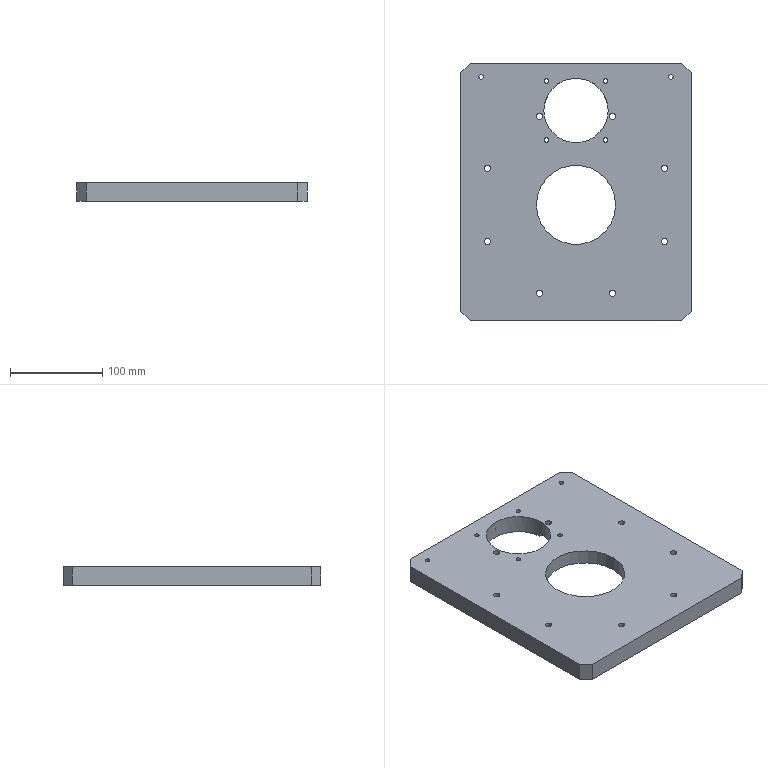Part | SolidWorks | features HoleWzd 4, Chamfer 1, Extrusion 1, ICE 1 | 1 solid | 50 faces | box 250 x 280 x 20 mm | volume 1073661 mm3 | cylinder 37 | plane 11 | cone 2 | commonest cylinder face diameters 6.8 x16 5 x14 222 x3 70 x2 86 x2